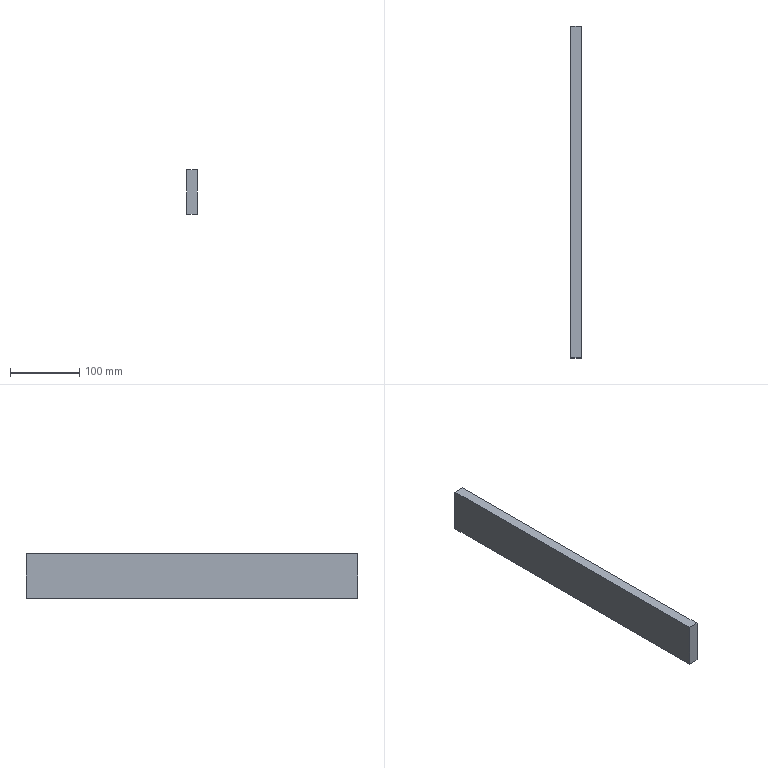Part | STEP file | Superstructure_3_1 | 1 solid | 6 faces | box 15 x 480 x 65 mm | volume 468000 mm3 | plane 6
STEP:
#1=CARTESIAN_POINT('',(0.,0.,0.));
#2=DIRECTION('',(0.,0.,1.));
#3=DIRECTION('',(1.,0.,0.));
#4=AXIS2_PLACEMENT_3D('',#1,#2,#3);
#5=CARTESIAN_POINT('',(-7.5,240.,32.5));
#6=VERTEX_POINT('',#5);
#7=CARTESIAN_POINT('',(-7.5,-240.,32.5));
#8=VERTEX_POINT('',#7);
#9=CARTESIAN_POINT('',(-7.5,240.,32.5));
#10=DIRECTION('',(0.,-1.,0.));
#11=VECTOR('',#10,1.);
#12=LINE('',#9,#11);
#13=CARTESIAN_POINT('',(-7.5,240.,32.5));
#14=DIRECTION('',(1.,0.,0.));
#15=DIRECTION('',(0.,0.,-1.));
#16=AXIS2_PLACEMENT_3D('',#13,#14,#15);
#17=PLANE('',#16);
#18=CARTESIAN_POINT('',(0.,0.));
#19=DIRECTION('',(0.,-1.));
#20=VECTOR('',#19,1.);
#21=LINE('',#18,#20);
#22=(GEOMETRIC_REPRESENTATION_CONTEXT(2)PARAMETRIC_REPRESENTATION_CONTEXT()REPRESENTATION_CONTEXT('',''));
#23=DEFINITIONAL_REPRESENTATION('',(#21),#22);
#24=PCURVE('',#17,#23);
#25=CARTESIAN_POINT('',(7.5,240.,32.5));
#26=DIRECTION('',(0.,0.,-1.));
#27=DIRECTION('',(-1.,0.,0.));
#28=AXIS2_PLACEMENT_3D('',#25,#26,#27);
#29=PLANE('',#28);
#30=CARTESIAN_POINT('',(15.,0.));
#31=DIRECTION('',(0.,-1.));
#32=VECTOR('',#31,1.);
#33=LINE('',#30,#32);
#34=(GEOMETRIC_REPRESENTATION_CONTEXT(2)PARAMETRIC_REPRESENTATION_CONTEXT()REPRESENTATION_CONTEXT('',''));
#35=DEFINITIONAL_REPRESENTATION('',(#33),#34);
#36=PCURVE('',#29,#35);
#37=SURFACE_CURVE('',#12,(#24,#36),.PCURVE_S1.);
#38=EDGE_CURVE('',#6,#8,#37,.T.);
#39=ORIENTED_EDGE('',*,*,#38,.T.);
#40=CARTESIAN_POINT('',(-7.5,-240.,-32.5));
#41=VERTEX_POINT('',#40);
#42=CARTESIAN_POINT('',(-7.5,-240.,32.5));
#43=DIRECTION('',(0.,0.,-1.));
#44=VECTOR('',#43,1.);
#45=LINE('',#42,#44);
#46=CARTESIAN_POINT('',(0.,-480.));
#47=DIRECTION('',(1.,0.));
#48=VECTOR('',#47,1.);
#49=LINE('',#46,#48);
#50=(GEOMETRIC_REPRESENTATION_CONTEXT(2)PARAMETRIC_REPRESENTATION_CONTEXT()REPRESENTATION_CONTEXT('',''));
#51=DEFINITIONAL_REPRESENTATION('',(#49),#50);
#52=PCURVE('',#17,#51);
#53=CARTESIAN_POINT('',(0.,-240.,0.));
#54=DIRECTION('',(0.,1.,0.));
#55=DIRECTION('',(0.,0.,1.));
#56=AXIS2_PLACEMENT_3D('',#53,#54,#55);
#57=PLANE('',#56);
#58=CARTESIAN_POINT('',(32.5,-7.5));
#59=DIRECTION('',(-1.,0.));
#60=VECTOR('',#59,1.);
#61=LINE('',#58,#60);
#62=(GEOMETRIC_REPRESENTATION_CONTEXT(2)PARAMETRIC_REPRESENTATION_CONTEXT()REPRESENTATION_CONTEXT('',''));
#63=DEFINITIONAL_REPRESENTATION('',(#61),#62);
#64=PCURVE('',#57,#63);
#65=SURFACE_CURVE('',#45,(#52,#64),.PCURVE_S1.);
#66=EDGE_CURVE('',#8,#41,#65,.T.);
#67=ORIENTED_EDGE('',*,*,#66,.T.);
#68=CARTESIAN_POINT('',(-7.5,240.,-32.5));
#69=VERTEX_POINT('',#68);
#70=CARTESIAN_POINT('',(-7.5,240.,-32.5));
#71=DIRECTION('',(0.,-1.,0.));
#72=VECTOR('',#71,1.);
#73=LINE('',#70,#72);
#74=CARTESIAN_POINT('',(65.,0.));
#75=DIRECTION('',(0.,-1.));
#76=VECTOR('',#75,1.);
#77=LINE('',#74,#76);
#78=(GEOMETRIC_REPRESENTATION_CONTEXT(2)PARAMETRIC_REPRESENTATION_CONTEXT()REPRESENTATION_CONTEXT('',''));
#79=DEFINITIONAL_REPRESENTATION('',(#77),#78);
#80=PCURVE('',#17,#79);
#81=CARTESIAN_POINT('',(-7.5,240.,-32.5));
#82=DIRECTION('',(0.,0.,1.));
#83=DIRECTION('',(1.,0.,0.));
#84=AXIS2_PLACEMENT_3D('',#81,#82,#83);
#85=PLANE('',#84);
#86=CARTESIAN_POINT('',(0.,0.));
#87=DIRECTION('',(0.,-1.));
#88=VECTOR('',#87,1.);
#89=LINE('',#86,#88);
#90=(GEOMETRIC_REPRESENTATION_CONTEXT(2)PARAMETRIC_REPRESENTATION_CONTEXT()REPRESENTATION_CONTEXT('',''));
#91=DEFINITIONAL_REPRESENTATION('',(#89),#90);
#92=PCURVE('',#85,#91);
#93=SURFACE_CURVE('',#73,(#80,#92),.PCURVE_S1.);
#94=EDGE_CURVE('',#69,#41,#93,.T.);
#95=ORIENTED_EDGE('',*,*,#94,.F.);
#96=CARTESIAN_POINT('',(-7.5,240.,32.5));
#97=DIRECTION('',(0.,0.,-1.));
#98=VECTOR('',#97,1.);
#99=LINE('',#96,#98);
#100=CARTESIAN_POINT('',(0.,0.));
#101=DIRECTION('',(1.,0.));
#102=VECTOR('',#101,1.);
#103=LINE('',#100,#102);
#104=(GEOMETRIC_REPRESENTATION_CONTEXT(2)PARAMETRIC_REPRESENTATION_CONTEXT()REPRESENTATION_CONTEXT('',''));
#105=DEFINITIONAL_REPRESENTATION('',(#103),#104);
#106=PCURVE('',#17,#105);
#107=CARTESIAN_POINT('',(0.,240.,0.));
#108=DIRECTION('',(0.,1.,0.));
#109=DIRECTION('',(0.,0.,1.));
#110=AXIS2_PLACEMENT_3D('',#107,#108,#109);
#111=PLANE('',#110);
#112=CARTESIAN_POINT('',(32.5,-7.5));
#113=DIRECTION('',(-1.,0.));
#114=VECTOR('',#113,1.);
#115=LINE('',#112,#114);
#116=(GEOMETRIC_REPRESENTATION_CONTEXT(2)PARAMETRIC_REPRESENTATION_CONTEXT()REPRESENTATION_CONTEXT('',''));
#117=DEFINITIONAL_REPRESENTATION('',(#115),#116);
#118=PCURVE('',#111,#117);
#119=SURFACE_CURVE('',#99,(#106,#118),.PCURVE_S1.);
#120=EDGE_CURVE('',#6,#69,#119,.T.);
#121=ORIENTED_EDGE('',*,*,#120,.F.);
#122=EDGE_LOOP('',(#39,#67,#95,#121));
#123=FACE_BOUND('',#122,.F.);
#124=ADVANCED_FACE('',(#123),#17,.F.);
#125=ORIENTED_EDGE('',*,*,#94,.T.);
#126=CARTESIAN_POINT('',(7.5,-240.,-32.5));
#127=VERTEX_POINT('',#126);
#128=CARTESIAN_POINT('',(-7.5,-240.,-32.5));
#129=DIRECTION('',(1.,0.,0.));
#130=VECTOR('',#129,1.);
#131=LINE('',#128,#130);
#132=CARTESIAN_POINT('',(0.,-480.));
#133=DIRECTION('',(1.,0.));
#134=VECTOR('',#133,1.);
#135=LINE('',#132,#134);
#136=(GEOMETRIC_REPRESENTATION_CONTEXT(2)PARAMETRIC_REPRESENTATION_CONTEXT()REPRESENTATION_CONTEXT('',''));
#137=DEFINITIONAL_REPRESENTATION('',(#135),#136);
#138=PCURVE('',#85,#137);
#139=CARTESIAN_POINT('',(-32.5,-7.5));
#140=DIRECTION('',(0.,1.));
#141=VECTOR('',#140,1.);
#142=LINE('',#139,#141);
#143=(GEOMETRIC_REPRESENTATION_CONTEXT(2)PARAMETRIC_REPRESENTATION_CONTEXT()REPRESENTATION_CONTEXT('',''));
#144=DEFINITIONAL_REPRESENTATION('',(#142),#143);
#145=PCURVE('',#57,#144);
#146=SURFACE_CURVE('',#131,(#138,#145),.PCURVE_S1.);
#147=EDGE_CURVE('',#41,#127,#146,.T.);
#148=ORIENTED_EDGE('',*,*,#147,.T.);
#149=CARTESIAN_POINT('',(7.5,240.,-32.5));
#150=VERTEX_POINT('',#149);
#151=CARTESIAN_POINT('',(7.5,240.,-32.5));
#152=DIRECTION('',(0.,-1.,0.));
#153=VECTOR('',#152,1.);
#154=LINE('',#151,#153);
#155=CARTESIAN_POINT('',(15.,0.));
#156=DIRECTION('',(0.,-1.));
#157=VECTOR('',#156,1.);
#158=LINE('',#155,#157);
#159=(GEOMETRIC_REPRESENTATION_CONTEXT(2)PARAMETRIC_REPRESENTATION_CONTEXT()REPRESENTATION_CONTEXT('',''));
#160=DEFINITIONAL_REPRESENTATION('',(#158),#159);
#161=PCURVE('',#85,#160);
#162=CARTESIAN_POINT('',(7.5,240.,-32.5));
#163=DIRECTION('',(-1.,0.,0.));
#164=DIRECTION('',(0.,0.,1.));
#165=AXIS2_PLACEMENT_3D('',#162,#163,#164);
#166=PLANE('',#165);
#167=CARTESIAN_POINT('',(0.,0.));
#168=DIRECTION('',(0.,-1.));
#169=VECTOR('',#168,1.);
#170=LINE('',#167,#169);
#171=(GEOMETRIC_REPRESENTATION_CONTEXT(2)PARAMETRIC_REPRESENTATION_CONTEXT()REPRESENTATION_CONTEXT('',''));
#172=DEFINITIONAL_REPRESENTATION('',(#170),#171);
#173=PCURVE('',#166,#172);
#174=SURFACE_CURVE('',#154,(#161,#173),.PCURVE_S1.);
#175=EDGE_CURVE('',#150,#127,#174,.T.);
#176=ORIENTED_EDGE('',*,*,#175,.F.);
#177=CARTESIAN_POINT('',(-7.5,240.,-32.5));
#178=DIRECTION('',(1.,0.,0.));
#179=VECTOR('',#178,1.);
#180=LINE('',#177,#179);
#181=CARTESIAN_POINT('',(0.,0.));
#182=DIRECTION('',(1.,0.));
#183=VECTOR('',#182,1.);
#184=LINE('',#181,#183);
#185=(GEOMETRIC_REPRESENTATION_CONTEXT(2)PARAMETRIC_REPRESENTATION_CONTEXT()REPRESENTATION_CONTEXT('',''));
#186=DEFINITIONAL_REPRESENTATION('',(#184),#185);
#187=PCURVE('',#85,#186);
#188=CARTESIAN_POINT('',(-32.5,-7.5));
#189=DIRECTION('',(0.,1.));
#190=VECTOR('',#189,1.);
#191=LINE('',#188,#190);
#192=(GEOMETRIC_REPRESENTATION_CONTEXT(2)PARAMETRIC_REPRESENTATION_CONTEXT()REPRESENTATION_CONTEXT('',''));
#193=DEFINITIONAL_REPRESENTATION('',(#191),#192);
#194=PCURVE('',#111,#193);
#195=SURFACE_CURVE('',#180,(#187,#194),.PCURVE_S1.);
#196=EDGE_CURVE('',#69,#150,#195,.T.);
#197=ORIENTED_EDGE('',*,*,#196,.F.);
#198=EDGE_LOOP('',(#125,#148,#176,#197));
#199=FACE_BOUND('',#198,.F.);
#200=ADVANCED_FACE('',(#199),#85,.F.);
#201=ORIENTED_EDGE('',*,*,#175,.T.);
#202=CARTESIAN_POINT('',(7.5,-240.,32.5));
#203=VERTEX_POINT('',#202);
#204=CARTESIAN_POINT('',(7.5,-240.,-32.5));
#205=DIRECTION('',(0.,0.,1.));
#206=VECTOR('',#205,1.);
#207=LINE('',#204,#206);
#208=CARTESIAN_POINT('',(0.,-480.));
#209=DIRECTION('',(1.,0.));
#210=VECTOR('',#209,1.);
#211=LINE('',#208,#210);
#212=(GEOMETRIC_REPRESENTATION_CONTEXT(2)PARAMETRIC_REPRESENTATION_CONTEXT()REPRESENTATION_CONTEXT('',''));
#213=DEFINITIONAL_REPRESENTATION('',(#211),#212);
#214=PCURVE('',#166,#213);
#215=CARTESIAN_POINT('',(-32.5,7.5));
#216=DIRECTION('',(1.,0.));
#217=VECTOR('',#216,1.);
#218=LINE('',#215,#217);
#219=(GEOMETRIC_REPRESENTATION_CONTEXT(2)PARAMETRIC_REPRESENTATION_CONTEXT()REPRESENTATION_CONTEXT('',''));
#220=DEFINITIONAL_REPRESENTATION('',(#218),#219);
#221=PCURVE('',#57,#220);
#222=SURFACE_CURVE('',#207,(#214,#221),.PCURVE_S1.);
#223=EDGE_CURVE('',#127,#203,#222,.T.);
#224=ORIENTED_EDGE('',*,*,#223,.T.);
#225=CARTESIAN_POINT('',(7.5,240.,32.5));
#226=VERTEX_POINT('',#225);
#227=CARTESIAN_POINT('',(7.5,240.,32.5));
#228=DIRECTION('',(0.,-1.,0.));
#229=VECTOR('',#228,1.);
#230=LINE('',#227,#229);
#231=CARTESIAN_POINT('',(65.,0.));
#232=DIRECTION('',(0.,-1.));
#233=VECTOR('',#232,1.);
#234=LINE('',#231,#233);
#235=(GEOMETRIC_REPRESENTATION_CONTEXT(2)PARAMETRIC_REPRESENTATION_CONTEXT()REPRESENTATION_CONTEXT('',''));
#236=DEFINITIONAL_REPRESENTATION('',(#234),#235);
#237=PCURVE('',#166,#236);
#238=CARTESIAN_POINT('',(0.,0.));
#239=DIRECTION('',(0.,-1.));
#240=VECTOR('',#239,1.);
#241=LINE('',#238,#240);
#242=(GEOMETRIC_REPRESENTATION_CONTEXT(2)PARAMETRIC_REPRESENTATION_CONTEXT()REPRESENTATION_CONTEXT('',''));
#243=DEFINITIONAL_REPRESENTATION('',(#241),#242);
#244=PCURVE('',#29,#243);
#245=SURFACE_CURVE('',#230,(#237,#244),.PCURVE_S1.);
#246=EDGE_CURVE('',#226,#203,#245,.T.);
#247=ORIENTED_EDGE('',*,*,#246,.F.);
#248=CARTESIAN_POINT('',(7.5,240.,-32.5));
#249=DIRECTION('',(0.,0.,1.));
#250=VECTOR('',#249,1.);
#251=LINE('',#248,#250);
#252=CARTESIAN_POINT('',(0.,0.));
#253=DIRECTION('',(1.,0.));
#254=VECTOR('',#253,1.);
#255=LINE('',#252,#254);
#256=(GEOMETRIC_REPRESENTATION_CONTEXT(2)PARAMETRIC_REPRESENTATION_CONTEXT()REPRESENTATION_CONTEXT('',''));
#257=DEFINITIONAL_REPRESENTATION('',(#255),#256);
#258=PCURVE('',#166,#257);
#259=CARTESIAN_POINT('',(-32.5,7.5));
#260=DIRECTION('',(1.,0.));
#261=VECTOR('',#260,1.);
#262=LINE('',#259,#261);
#263=(GEOMETRIC_REPRESENTATION_CONTEXT(2)PARAMETRIC_REPRESENTATION_CONTEXT()REPRESENTATION_CONTEXT('',''));
#264=DEFINITIONAL_REPRESENTATION('',(#262),#263);
#265=PCURVE('',#111,#264);
#266=SURFACE_CURVE('',#251,(#258,#265),.PCURVE_S1.);
#267=EDGE_CURVE('',#150,#226,#266,.T.);
#268=ORIENTED_EDGE('',*,*,#267,.F.);
#269=EDGE_LOOP('',(#201,#224,#247,#268));
#270=FACE_BOUND('',#269,.F.);
#271=ADVANCED_FACE('',(#270),#166,.F.);
#272=ORIENTED_EDGE('',*,*,#246,.T.);
#273=CARTESIAN_POINT('',(7.5,-240.,32.5));
#274=DIRECTION('',(-1.,0.,0.));
#275=VECTOR('',#274,1.);
#276=LINE('',#273,#275);
#277=CARTESIAN_POINT('',(0.,-480.));
#278=DIRECTION('',(1.,0.));
#279=VECTOR('',#278,1.);
#280=LINE('',#277,#279);
#281=(GEOMETRIC_REPRESENTATION_CONTEXT(2)PARAMETRIC_REPRESENTATION_CONTEXT()REPRESENTATION_CONTEXT('',''));
#282=DEFINITIONAL_REPRESENTATION('',(#280),#281);
#283=PCURVE('',#29,#282);
#284=CARTESIAN_POINT('',(32.5,7.5));
#285=DIRECTION('',(0.,-1.));
#286=VECTOR('',#285,1.);
#287=LINE('',#284,#286);
#288=(GEOMETRIC_REPRESENTATION_CONTEXT(2)PARAMETRIC_REPRESENTATION_CONTEXT()REPRESENTATION_CONTEXT('',''));
#289=DEFINITIONAL_REPRESENTATION('',(#287),#288);
#290=PCURVE('',#57,#289);
#291=SURFACE_CURVE('',#276,(#283,#290),.PCURVE_S1.);
#292=EDGE_CURVE('',#203,#8,#291,.T.);
#293=ORIENTED_EDGE('',*,*,#292,.T.);
#294=ORIENTED_EDGE('',*,*,#38,.F.);
#295=CARTESIAN_POINT('',(7.5,240.,32.5));
#296=DIRECTION('',(-1.,0.,0.));
#297=VECTOR('',#296,1.);
#298=LINE('',#295,#297);
#299=CARTESIAN_POINT('',(0.,0.));
#300=DIRECTION('',(1.,0.));
#301=VECTOR('',#300,1.);
#302=LINE('',#299,#301);
#303=(GEOMETRIC_REPRESENTATION_CONTEXT(2)PARAMETRIC_REPRESENTATION_CONTEXT()REPRESENTATION_CONTEXT('',''));
#304=DEFINITIONAL_REPRESENTATION('',(#302),#303);
#305=PCURVE('',#29,#304);
#306=CARTESIAN_POINT('',(32.5,7.5));
#307=DIRECTION('',(0.,-1.));
#308=VECTOR('',#307,1.);
#309=LINE('',#306,#308);
#310=(GEOMETRIC_REPRESENTATION_CONTEXT(2)PARAMETRIC_REPRESENTATION_CONTEXT()REPRESENTATION_CONTEXT('',''));
#311=DEFINITIONAL_REPRESENTATION('',(#309),#310);
#312=PCURVE('',#111,#311);
#313=SURFACE_CURVE('',#298,(#305,#312),.PCURVE_S1.);
#314=EDGE_CURVE('',#226,#6,#313,.T.);
#315=ORIENTED_EDGE('',*,*,#314,.F.);
#316=EDGE_LOOP('',(#272,#293,#294,#315));
#317=FACE_BOUND('',#316,.F.);
#318=ADVANCED_FACE('',(#317),#29,.F.);
#319=ORIENTED_EDGE('',*,*,#120,.T.);
#320=ORIENTED_EDGE('',*,*,#196,.T.);
#321=ORIENTED_EDGE('',*,*,#267,.T.);
#322=ORIENTED_EDGE('',*,*,#314,.T.);
#323=EDGE_LOOP('',(#319,#320,#321,#322));
#324=FACE_BOUND('',#323,.F.);
#325=ADVANCED_FACE('',(#324),#111,.T.);
#326=ORIENTED_EDGE('',*,*,#66,.T.);
#327=ORIENTED_EDGE('',*,*,#147,.T.);
#328=ORIENTED_EDGE('',*,*,#223,.T.);
#329=ORIENTED_EDGE('',*,*,#292,.T.);
#330=EDGE_LOOP('',(#326,#327,#328,#329));
#331=FACE_BOUND('',#330,.T.);
#332=ADVANCED_FACE('',(#331),#57,.F.);
#333=CLOSED_SHELL('',(#124,#200,#271,#318,#325,#332));
#334=MANIFOLD_SOLID_BREP('',#333);
#335=(LENGTH_UNIT()NAMED_UNIT(*)SI_UNIT(.MILLI.,.METRE.));
#336=UNCERTAINTY_MEASURE_WITH_UNIT(LENGTH_MEASURE(0.0000001),#335,'','');
#337=(NAMED_UNIT(*)PLANE_ANGLE_UNIT()SI_UNIT($,.RADIAN.));
#338=(NAMED_UNIT(*)SI_UNIT($,.STERADIAN.)SOLID_ANGLE_UNIT());
#339=(GEOMETRIC_REPRESENTATION_CONTEXT(3)GLOBAL_UNCERTAINTY_ASSIGNED_CONTEXT((#336))GLOBAL_UNIT_ASSIGNED_CONTEXT((#335,#337,#338))REPRESENTATION_CONTEXT('',''));
#340=ADVANCED_BREP_SHAPE_REPRESENTATION('',(#4,#334),#339);